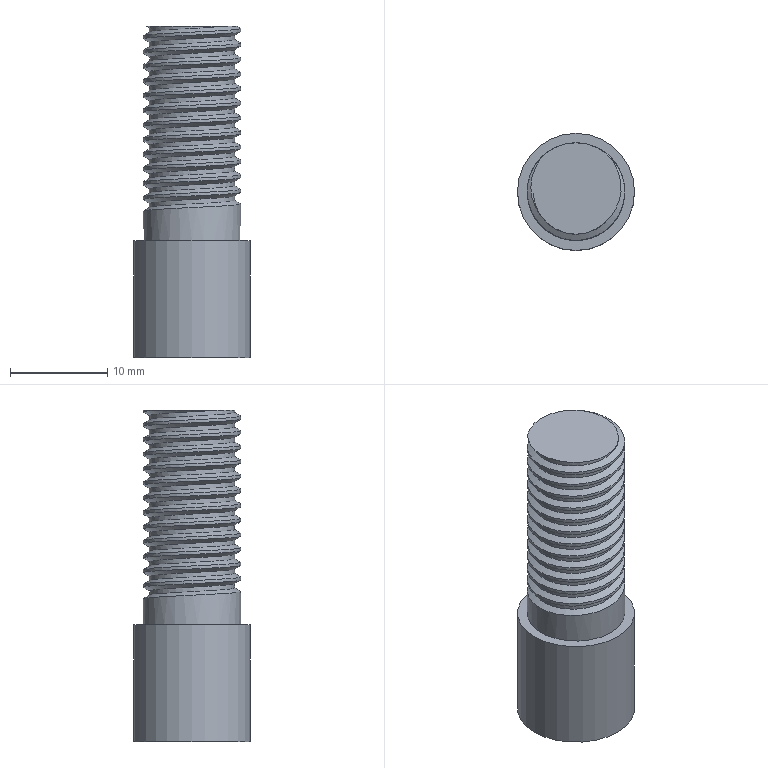Part | NX | features solid 2 | 1 solid | 22 faces | box 12 x 12 x 34 mm | volume 2866 mm3 | cylinder 16 | plane 4 | spline 2 | commonest cylinder face diameters 10 x14 8.75 x1 12 x1